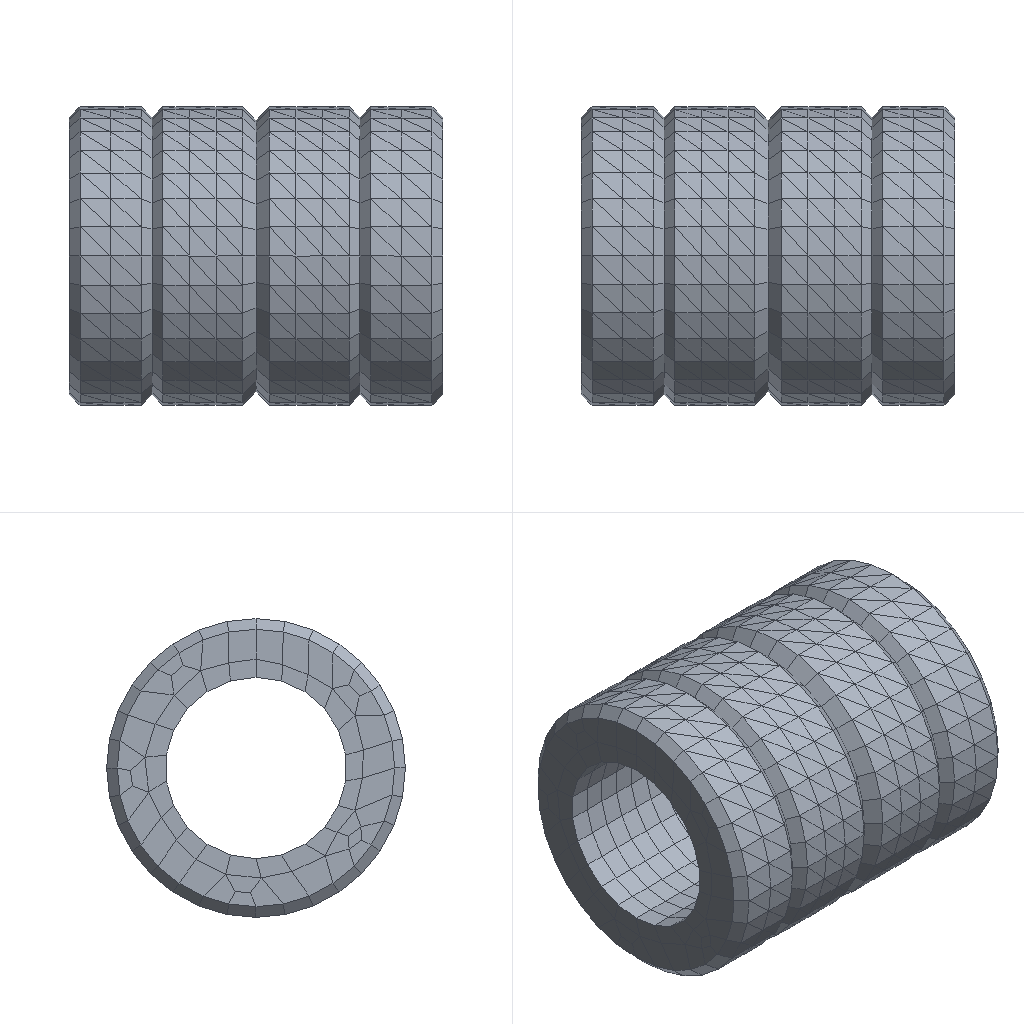Simulation study | ansys workbench
Ansys APDL input file, long lists of numbers shortened:
/batch
/config,noeldb,1     ! force off writing results to database
*get,_wallstrt,active,,time,wall
! ANSYS input file written by Workbench version 2022 R1
! File used for geometry attach: F:\ansys（分析文件汇总)\胶桶有限元分析\卡瓦仿真.STEP
/title,fenc--____ (B5)
! ****** Begin Custom Load Command Snippet ******
/COM, ACT Extensions:
/COM,     LSDYNA, 2021.1
/COM,
! ****** End   Custom Load Command Snippet ******
*DIM,_wb_ProjectScratch_dir,string,248
_wb_ProjectScratch_dir(1) = 'F:\ansys（分析文件汇总)\胶桶有限元分析\_ProjectScratch\Scr3E1A\'
*DIM,_wb_SolverFiles_dir,string,248
_wb_SolverFiles_dir(1) = 'F:\ansys（分析文件汇总)\胶桶有限元分析\fenc_files\dp0\SYS-1\MECH\'
*DIM,_wb_userfiles_dir,string,248
_wb_userfiles_dir(1) = 'F:\ansys（分析文件汇总)\胶桶有限元分析\fenc_files\user_files\'
/com,--- Data in consistent NMM units. See Solving Units in the help system for more information.
/units,MPA
/nopr
/wb,file,start              !  signify a WB generated input file
/prep7
! Turn off shape checking because checks already performed inside WB mesher.
! See help system for more information.
SHPP,OFF,,NOWARN
/nolist
etcon,set             ! allow ANSYS to choose best KEYOP's for 180x elements, resets any applicable keyopt to MAPDL defaults
/com,*********** Nodes for the whole assembly ***********
nblock,3,,6278
(1i9,3e20.9e3)
        1     2.415535804E+01     1.493952260E+01     1.131000000E+02
! (5707 more lines like these left out)
-1
/wb,elem,start            !  set before creation of elements
/com,*********** Elements for Body 1 "________|____(____)1" ***********
et,1,186
keyo,1,2,1          ! set full integration on SOLID186
eblock,19,solid,,692
(19i9)
        1        1        1        1        0        0        0        0       20        0      301     1783     1984     1951     1921     2298     2231     2242     2252
! (1383 more lines like these left out)
-1
/com,*********** Elements for Body 2 "____|____-____1" ***********
et,2,186
keyo,2,2,1          ! set full integration on SOLID186
eblock,19,solid,,300
(19i9)
        2        2        2        2        0        0        0        0       20        0        1        1      373      386      448      228      384      385      486
! (599 more lines like these left out)
-1
/wb,elem,end               !  done creating elements
/com,*********** Send User Defined Coordinate System(s) ***********
csys,0
toffst,273.15,  ! Temperature offset from absolute zero
/com,*********** Set Reference Temperature ***********
tref,22.
/wb,mat,start              !  starting to send materials
/com,*********** Send Materials ***********
Temperature = 'TEMP' ! Temperature
MP,DENS,1,7.85e-09,	! tonne mm^-3
MP,ALPX,1,1.2e-05,	! C^-1
MP,C,1,434000000,	! mm^2 s^-2 C^-1
MP,KXX,1,60.5,	! tonne mm s^-3 C^-1
MP,RSVX,1,0.00017,	! ohm mm
MP,EX,1,200000,	! tonne s^-2 mm^-1
MP,NUXY,1,0.3,
MP,MURX,1,10000,
Temperature = 'TEMP' ! Temperature
MP,DENS,2,7.85e-09,	! tonne mm^-3
MP,ALPX,2,1.2e-05,	! C^-1
MP,C,2,434000000,	! mm^2 s^-2 C^-1
MP,KXX,2,60.5,	! tonne mm s^-3 C^-1
MP,RSVX,2,0.00017,	! ohm mm
MP,EX,2,200000,	! tonne s^-2 mm^-1
MP,NUXY,2,0.3,
MP,MURX,2,10000,
/wb,mat,end                !  done sending materials
!************************* Model Summary ********************
!________|____(____)1,	结构钢,	matid,	1
!____|____-____1,	结构钢,	matid,	2
!************************* End Model Summary ********************
! get the diagonal of the bounding box. Needed later for other things
*get,_xmin,node,,mnloc,x
*get,_ymin,node,,mnloc,y
*get,_zmin,node,,mnloc,z
*get,_xmax,node,,mxloc,x
*get,_ymax,node,,mxloc,y
*get,_zmax,node,,mxloc,z
_ASMDIAG=(_xmax-_xmin)*(_xmax-_xmin)+(_ymax-_ymin)*(_ymax-_ymin)+(_zmax-_zmin)*(_zmax-_zmin)
_ASMDIAG=SQRT(_ASMDIAG)
/wb,contact,start          !  starting to send contact
/com,*********** Create Contact "摩擦的 - ____|____-____1 至 ________|____(____)1" ***********
/com,            Real Constant Set For Above Contact Is 4 & 3
*set,tid,4
*set,cid,3
r,tid
r,cid
et,tid,170
et,cid,174
eblock,10,,,100
(15i9)
     2049        4        4        4        0      344      229      305      343     1261     1260     1434     1511
! (99 more lines like these left out)
-1
eblock,10,,,100
(15i9)
     2149        3        3        3        0      344      229      305      343     1261     1260     1434     1511
! (99 more lines like these left out)
-1
eblock,10,,,24
(15i9)
     2249        3        4        3        0     2785     2429     2428     2784     4904     4899     4901     5615
! (23 more lines like these left out)
-1
eblock,10,,,24
(15i9)
     2273        4        3        4        0     2785     2429     2428     2784     4904     4899     4901     5615
! (23 more lines like these left out)
-1
keyo,cid,8,2               ! auto create asymmetric contact (from Program Controlled setting)
keyo,cid,10,0              ! adjust contact stiffness each NR iteration (from Program Controlled setting)
keyo,cid,12,0              ! standard contact
mp,mu,cid,0.2       ! unitless
keyo,cid,18,1              ! small sliding turned on by application
keyo,cid,2,0               ! augmented Lagrange (from Program Controlled setting)
keyo,cid,4,0               ! on Gauss point (from Program Controlled setting)
keyo,cid,9,0               ! use real geometry with stepped effects
keyo,cid,7,0               ! No Prediction
rmod,tid,3,1.       ! FKN
rmod,tid,5,0.       ! ICONT
rmod,tid,6,0.       ! PINB
rmod,tid,10,0.      ! CNOF
rmod,tid,12,0.      ! FKT
rmod,tid,36,50      ! WB DSID
rmod,cid,3,1.       ! FKN
rmod,cid,5,0.       ! ICONT
rmod,cid,6,0.       ! PINB
rmod,cid,10,0.      ! CNOF
rmod,cid,12,0.      ! FKT
rmod,cid,36,50      ! WB DSID
nsel,all
esel,all
/wb,contact,end            !  done creating contacts
/golist
/wb,load,start             !  starting to send loads
/com,*********** Fixed Supports ***********
CMBLOCK,_FIXEDSU,NODE,      444
(8i10)
       153       154       155       156       157       158       159       160
! (55 more lines like these left out)
cmsel,s,_FIXEDSU
d,all,all
nsel,all
/com,*********** Define Force Using Surface Effect Elements ***********
local,12,0,0.,0.,0.,0.,0.,0.
csys,0
et,5,154
eblock,10,,,76
(15i9)
     2297        5        5        5       12     2785     2429     2428     2784     4904     4899     4901     5615
! (75 more lines like these left out)
-1
esel,s,type,,5
keyop,5,2,1                ! Apply load in local coordinate system
keyop,5,7,1                ! Use original area so load is constant in large deformation
esel,all
/com,*********** Define Force Using Surface Effect Elements ***********
local,13,0,0.,0.,0.,0.,0.,0.
csys,0
et,6,154
eblock,10,,,100
(15i9)
     2373        6        6        6       13      344      229      305      343     1261     1260     1434     1511
! (99 more lines like these left out)
-1
esel,s,type,,6
keyop,6,2,1                ! Apply load in local coordinate system
keyop,6,7,1                ! Use original area so load is constant in large deformation
esel,all
/gst,on,on
fini
*get,_numnode,node,0,count
*get,_numelem,elem,0,count
*get, _MAXELEMNUM, elem, 0, NUM, MAX
*get, _MAXNODENUM, node, 0, NUM, MAX
*get, _MAXELEMTYPE, etyp, 0, NUM, MAX
*get, _MAXREALCONST, real, 0, NUM, MAX
/go
/wb,load,end               !  done creating loads
/com,--- Number of total nodes = %_numnode%
/com,--- Number of contact elements = 424
/com,--- Number of spring elements = 0
/com,--- Number of bearing elements = 0
/com,--- Number of solid elements = 992
/com,--- Number of condensed parts = 0
/com,--- Number of total elements = %_numelem%
*get,_wallbsol,active,,time,wall
/com,****************************************************************************
/com,*************************    SOLUTION       ********************************
/com,****************************************************************************
/solu
antype,0                   ! static analysis
_thickRatio=  1     ! Ratio of thick parts in the model
eqsl,pcg,1e-8,,,,,,1
cntr,print,1               ! print out contact info and also make no initial contact an error
dmpoption,emat,no             ! Don't combine emat file for DANSYS
dmpoption,esav,no             ! Don't combine esav file for DANSYS
nldiag,cont,iter           ! print out contact info each equilibrium iteration
rescontrol,define,last,last,,dele	   ! Program Controlled
/com,****************************************************
/com,******************* SOLVE FOR LS 1 OF 1 ****************
esel,s,type,,5
nsle
sfe,all,1,pres,1,-1054.457
sfe,all,2,pres,1,1.06035457494494e-012
sfe,all,3,pres,1,0.
esel,s,type,,6
nsle
sfe,all,1,pres,1,0.
sfe,all,2,pres,1,2.786
sfe,all,3,pres,1,0.
nsel,all
esel,all
/nopr
/gopr
autots,on                  ! Workbench Program Controlled automatic time stepping
nsub,1,10,1                ! due to presence of general nonlinear
time,1.
outres,erase
outres,all,none
outres,nsol,all,
outres,rsol,all
outres,eangl,all
outres,etmp,all
outres,veng,all
outres,strs,all,
outres,epel,all,
outres,eppl,all,
outres,cont,all,
! *********** WB SOLVE COMMAND ***********
! check interactive state
*get,ANSINTER_,active,,int
*if,ANSINTER_,ne,0,then
/eof
*endif
solve
/com *************** Write FE CONNECTORS *********
CEWRITE,file,ce,,INTE
/com,****************************************************
/com,*************** FINISHED SOLVE FOR LS 1 *************
*get,_wallasol,active,,time,wall
/nopr
*get,_numnode,node,0,count
*get,_numelem,elem,0,count
*get, _MAXELEMNUM, elem, 0, NUM, MAX
*get, _MAXNODENUM, node, 0, NUM, MAX,,,INTERNAL
*get, _MAXELEMTYPE, etyp, 0, NUM, MAX
*get, _MAXREALCONST, real, 0, NUM, MAX
/gopr
*get,_PCGITER,active,,solu,cgiter
/post1
xmlo,ENCODING,ISO-8859-1
xmlo,parm
/xml,parm,xml
fini
/gopr
*get,_walldone,active,,time,wall
_preptime=(_wallbsol-_wallstrt)*3600
_solvtime=(_wallasol-_wallbsol)*3600
_posttime=(_walldone-_wallasol)*3600
_totaltim=(_walldone-_wallstrt)*3600
*get,_dlbratio,active,0,solu,dlbr
*get,_combtime,active,0,solu,comb
*get,_ssmode,active,0,solu,ssmm
*get,_ndofs,active,0,solu,ndof
*get,_sol_end_time,active,0,set,time
*if,_sol_end_time,eq,1.,then
/fclean				!clean distributed files
*endif
/com,--- Total number of nodes = %_numnode%
/com,--- Total number of elements = %_numelem%
/com,--- Element load balance ratio = %_dlbratio%
/com,--- Time to combine distributed files = %_combtime%
/com,--- Sparse memory mode = %_ssmode%
/com,--- Number of DOF = %_ndofs%
/wb,file,end               ! done with WB generated input